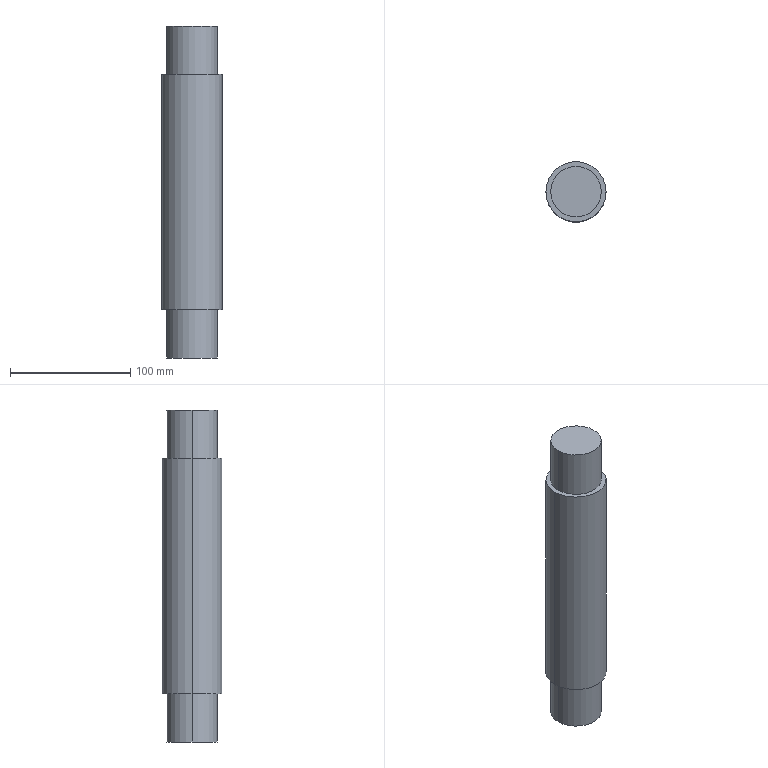Part | SolidWorks | features Extrusion 1, ICE 1, MirrorPattern 1 | 1 solid | 10 faces | box 50 x 50 x 276 mm | volume 495680 mm3 | cylinder 6 | plane 4 | commonest cylinder face diameters 42 x4 50 x2
STEP:
#1=CARTESIAN_POINT('',(21.,0.,-138.));
#2=VERTEX_POINT('',#1);
#3=CARTESIAN_POINT('',(-21.,0.,-138.));
#4=VERTEX_POINT('',#3);
#5=CARTESIAN_POINT('',(0.,0.,-138.));
#6=DIRECTION('',(0.,0.,1.));
#7=DIRECTION('',(1.,0.,0.));
#8=AXIS2_PLACEMENT_3D('',#5,#6,#7);
#9=CIRCLE('',#8,21.);
#10=EDGE_CURVE('',#2,#4,#9,.T.);
#11=ORIENTED_EDGE('',*,*,#10,.T.);
#12=CARTESIAN_POINT('',(-21.,0.,-98.));
#13=VERTEX_POINT('',#12);
#14=CARTESIAN_POINT('',(-21.,0.,-138.));
#15=DIRECTION('',(0.,0.,1.));
#16=VECTOR('',#15,1000.);
#17=LINE('',#14,#16);
#18=EDGE_CURVE('',#4,#13,#17,.T.);
#19=ORIENTED_EDGE('',*,*,#18,.T.);
#20=CARTESIAN_POINT('',(21.,0.,-98.));
#21=VERTEX_POINT('',#20);
#22=CARTESIAN_POINT('',(0.,0.,-98.));
#23=DIRECTION('',(0.,0.,1.));
#24=DIRECTION('',(1.,0.,0.));
#25=AXIS2_PLACEMENT_3D('',#22,#23,#24);
#26=CIRCLE('',#25,21.);
#27=EDGE_CURVE('',#21,#13,#26,.T.);
#28=ORIENTED_EDGE('',*,*,#27,.F.);
#29=CARTESIAN_POINT('',(21.,0.,-138.));
#30=DIRECTION('',(0.,0.,1.));
#31=VECTOR('',#30,1000.);
#32=LINE('',#29,#31);
#33=EDGE_CURVE('',#2,#21,#32,.T.);
#34=ORIENTED_EDGE('',*,*,#33,.F.);
#35=EDGE_LOOP('',(#11,#19,#28,#34));
#36=FACE_OUTER_BOUND('',#35,.T.);
#37=CARTESIAN_POINT('',(0.,0.,-138.));
#38=DIRECTION('',(0.,0.,1.));
#39=DIRECTION('',(1.,0.,0.));
#40=AXIS2_PLACEMENT_3D('',#37,#38,#39);
#41=CYLINDRICAL_SURFACE('',#40,21.);
#42=ADVANCED_FACE('',(#36),#41,.T.);
#43=CARTESIAN_POINT('',(21.,0.,138.));
#44=VERTEX_POINT('',#43);
#45=CARTESIAN_POINT('',(-21.,0.,138.));
#46=VERTEX_POINT('',#45);
#47=CARTESIAN_POINT('',(0.,0.,138.));
#48=DIRECTION('',(0.,0.,1.));
#49=DIRECTION('',(1.,0.,0.));
#50=AXIS2_PLACEMENT_3D('',#47,#48,#49);
#51=CIRCLE('',#50,21.);
#52=EDGE_CURVE('',#44,#46,#51,.T.);
#53=ORIENTED_EDGE('',*,*,#52,.F.);
#54=CARTESIAN_POINT('',(21.,0.,98.));
#55=VERTEX_POINT('',#54);
#56=CARTESIAN_POINT('',(21.,0.,138.));
#57=DIRECTION('',(0.,0.,-1.));
#58=VECTOR('',#57,1000.);
#59=LINE('',#56,#58);
#60=EDGE_CURVE('',#44,#55,#59,.T.);
#61=ORIENTED_EDGE('',*,*,#60,.T.);
#62=CARTESIAN_POINT('',(-21.,0.,98.));
#63=VERTEX_POINT('',#62);
#64=CARTESIAN_POINT('',(0.,0.,98.));
#65=DIRECTION('',(0.,0.,1.));
#66=DIRECTION('',(1.,0.,0.));
#67=AXIS2_PLACEMENT_3D('',#64,#65,#66);
#68=CIRCLE('',#67,21.);
#69=EDGE_CURVE('',#55,#63,#68,.T.);
#70=ORIENTED_EDGE('',*,*,#69,.T.);
#71=CARTESIAN_POINT('',(-21.,0.,138.));
#72=DIRECTION('',(0.,0.,-1.));
#73=VECTOR('',#72,1000.);
#74=LINE('',#71,#73);
#75=EDGE_CURVE('',#46,#63,#74,.T.);
#76=ORIENTED_EDGE('',*,*,#75,.F.);
#77=EDGE_LOOP('',(#53,#61,#70,#76));
#78=FACE_OUTER_BOUND('',#77,.T.);
#79=CARTESIAN_POINT('',(0.,0.,138.));
#80=DIRECTION('',(0.,0.,-1.));
#81=DIRECTION('',(-1.,0.,0.));
#82=AXIS2_PLACEMENT_3D('',#79,#80,#81);
#83=CYLINDRICAL_SURFACE('',#82,21.);
#84=ADVANCED_FACE('',(#78),#83,.T.);
#85=CARTESIAN_POINT('',(25.,0.,98.));
#86=VERTEX_POINT('',#85);
#87=CARTESIAN_POINT('',(-25.,0.,98.));
#88=VERTEX_POINT('',#87);
#89=CARTESIAN_POINT('',(0.,0.,98.));
#90=DIRECTION('',(0.,0.,1.));
#91=DIRECTION('',(1.,0.,0.));
#92=AXIS2_PLACEMENT_3D('',#89,#90,#91);
#93=CIRCLE('',#92,25.);
#94=EDGE_CURVE('',#86,#88,#93,.T.);
#95=ORIENTED_EDGE('',*,*,#94,.F.);
#96=CARTESIAN_POINT('',(25.,0.,-98.));
#97=VERTEX_POINT('',#96);
#98=CARTESIAN_POINT('',(25.,0.,98.));
#99=DIRECTION('',(0.,0.,-1.));
#100=VECTOR('',#99,1000.);
#101=LINE('',#98,#100);
#102=EDGE_CURVE('',#86,#97,#101,.T.);
#103=ORIENTED_EDGE('',*,*,#102,.T.);
#104=CARTESIAN_POINT('',(-25.,0.,-98.));
#105=VERTEX_POINT('',#104);
#106=CARTESIAN_POINT('',(0.,0.,-98.));
#107=DIRECTION('',(0.,0.,1.));
#108=DIRECTION('',(1.,0.,0.));
#109=AXIS2_PLACEMENT_3D('',#106,#107,#108);
#110=CIRCLE('',#109,25.);
#111=EDGE_CURVE('',#97,#105,#110,.T.);
#112=ORIENTED_EDGE('',*,*,#111,.T.);
#113=CARTESIAN_POINT('',(-25.,0.,98.));
#114=DIRECTION('',(0.,0.,-1.));
#115=VECTOR('',#114,1000.);
#116=LINE('',#113,#115);
#117=EDGE_CURVE('',#88,#105,#116,.T.);
#118=ORIENTED_EDGE('',*,*,#117,.F.);
#119=EDGE_LOOP('',(#95,#103,#112,#118));
#120=FACE_OUTER_BOUND('',#119,.T.);
#121=CARTESIAN_POINT('',(0.,0.,98.));
#122=DIRECTION('',(0.,0.,-1.));
#123=DIRECTION('',(-1.,0.,0.));
#124=AXIS2_PLACEMENT_3D('',#121,#122,#123);
#125=CYLINDRICAL_SURFACE('',#124,25.);
#126=ADVANCED_FACE('',(#120),#125,.T.);
#127=ORIENTED_EDGE('',*,*,#102,.F.);
#128=CARTESIAN_POINT('',(0.,0.,98.));
#129=DIRECTION('',(0.,0.,1.));
#130=DIRECTION('',(1.,0.,0.));
#131=AXIS2_PLACEMENT_3D('',#128,#129,#130);
#132=CIRCLE('',#131,25.);
#133=EDGE_CURVE('',#88,#86,#132,.T.);
#134=ORIENTED_EDGE('',*,*,#133,.F.);
#135=ORIENTED_EDGE('',*,*,#117,.T.);
#136=CARTESIAN_POINT('',(0.,0.,-98.));
#137=DIRECTION('',(0.,0.,1.));
#138=DIRECTION('',(1.,0.,0.));
#139=AXIS2_PLACEMENT_3D('',#136,#137,#138);
#140=CIRCLE('',#139,25.);
#141=EDGE_CURVE('',#105,#97,#140,.T.);
#142=ORIENTED_EDGE('',*,*,#141,.T.);
#143=EDGE_LOOP('',(#127,#134,#135,#142));
#144=FACE_OUTER_BOUND('',#143,.T.);
#145=CARTESIAN_POINT('',(0.,0.,98.));
#146=DIRECTION('',(0.,0.,-1.));
#147=DIRECTION('',(-1.,0.,0.));
#148=AXIS2_PLACEMENT_3D('',#145,#146,#147);
#149=CYLINDRICAL_SURFACE('',#148,25.);
#150=ADVANCED_FACE('',(#144),#149,.T.);
#151=CARTESIAN_POINT('',(0.,0.,98.));
#152=DIRECTION('',(0.,0.,1.));
#153=DIRECTION('',(1.,0.,0.));
#154=AXIS2_PLACEMENT_3D('',#151,#152,#153);
#155=CIRCLE('',#154,21.);
#156=EDGE_CURVE('',#63,#55,#155,.T.);
#157=ORIENTED_EDGE('',*,*,#156,.F.);
#158=ORIENTED_EDGE('',*,*,#69,.F.);
#159=EDGE_LOOP('',(#157,#158));
#160=FACE_BOUND('',#159,.T.);
#161=ORIENTED_EDGE('',*,*,#133,.T.);
#162=ORIENTED_EDGE('',*,*,#94,.T.);
#163=EDGE_LOOP('',(#161,#162));
#164=FACE_OUTER_BOUND('',#163,.T.);
#165=CARTESIAN_POINT('',(0.,0.,98.));
#166=DIRECTION('',(0.,0.,1.));
#167=DIRECTION('',(1.,0.,0.));
#168=AXIS2_PLACEMENT_3D('',#165,#166,#167);
#169=PLANE('',#168);
#170=ADVANCED_FACE('',(#160,#164),#169,.T.);
#171=ORIENTED_EDGE('',*,*,#27,.T.);
#172=CARTESIAN_POINT('',(0.,0.,-98.));
#173=DIRECTION('',(0.,0.,1.));
#174=DIRECTION('',(1.,0.,0.));
#175=AXIS2_PLACEMENT_3D('',#172,#173,#174);
#176=CIRCLE('',#175,21.);
#177=EDGE_CURVE('',#13,#21,#176,.T.);
#178=ORIENTED_EDGE('',*,*,#177,.T.);
#179=EDGE_LOOP('',(#171,#178));
#180=FACE_BOUND('',#179,.T.);
#181=ORIENTED_EDGE('',*,*,#141,.F.);
#182=ORIENTED_EDGE('',*,*,#111,.F.);
#183=EDGE_LOOP('',(#181,#182));
#184=FACE_OUTER_BOUND('',#183,.T.);
#185=CARTESIAN_POINT('',(0.,0.,-98.));
#186=DIRECTION('',(0.,0.,1.));
#187=DIRECTION('',(1.,0.,0.));
#188=AXIS2_PLACEMENT_3D('',#185,#186,#187);
#189=PLANE('',#188);
#190=ADVANCED_FACE('',(#180,#184),#189,.F.);
#191=ORIENTED_EDGE('',*,*,#60,.F.);
#192=CARTESIAN_POINT('',(0.,0.,138.));
#193=DIRECTION('',(0.,0.,1.));
#194=DIRECTION('',(1.,0.,0.));
#195=AXIS2_PLACEMENT_3D('',#192,#193,#194);
#196=CIRCLE('',#195,21.);
#197=EDGE_CURVE('',#46,#44,#196,.T.);
#198=ORIENTED_EDGE('',*,*,#197,.F.);
#199=ORIENTED_EDGE('',*,*,#75,.T.);
#200=ORIENTED_EDGE('',*,*,#156,.T.);
#201=EDGE_LOOP('',(#191,#198,#199,#200));
#202=FACE_OUTER_BOUND('',#201,.T.);
#203=CARTESIAN_POINT('',(0.,0.,138.));
#204=DIRECTION('',(0.,0.,-1.));
#205=DIRECTION('',(-1.,0.,0.));
#206=AXIS2_PLACEMENT_3D('',#203,#204,#205);
#207=CYLINDRICAL_SURFACE('',#206,21.);
#208=ADVANCED_FACE('',(#202),#207,.T.);
#209=ORIENTED_EDGE('',*,*,#197,.T.);
#210=ORIENTED_EDGE('',*,*,#52,.T.);
#211=EDGE_LOOP('',(#209,#210));
#212=FACE_OUTER_BOUND('',#211,.T.);
#213=CARTESIAN_POINT('',(0.,0.,138.));
#214=DIRECTION('',(0.,0.,1.));
#215=DIRECTION('',(1.,0.,0.));
#216=AXIS2_PLACEMENT_3D('',#213,#214,#215);
#217=PLANE('',#216);
#218=ADVANCED_FACE('',(#212),#217,.T.);
#219=ORIENTED_EDGE('',*,*,#18,.F.);
#220=CARTESIAN_POINT('',(0.,0.,-138.));
#221=DIRECTION('',(0.,0.,1.));
#222=DIRECTION('',(1.,0.,0.));
#223=AXIS2_PLACEMENT_3D('',#220,#221,#222);
#224=CIRCLE('',#223,21.);
#225=EDGE_CURVE('',#4,#2,#224,.T.);
#226=ORIENTED_EDGE('',*,*,#225,.T.);
#227=ORIENTED_EDGE('',*,*,#33,.T.);
#228=ORIENTED_EDGE('',*,*,#177,.F.);
#229=EDGE_LOOP('',(#219,#226,#227,#228));
#230=FACE_OUTER_BOUND('',#229,.T.);
#231=CARTESIAN_POINT('',(0.,0.,-138.));
#232=DIRECTION('',(0.,0.,1.));
#233=DIRECTION('',(1.,0.,0.));
#234=AXIS2_PLACEMENT_3D('',#231,#232,#233);
#235=CYLINDRICAL_SURFACE('',#234,21.);
#236=ADVANCED_FACE('',(#230),#235,.T.);
#237=ORIENTED_EDGE('',*,*,#10,.F.);
#238=ORIENTED_EDGE('',*,*,#225,.F.);
#239=EDGE_LOOP('',(#237,#238));
#240=FACE_OUTER_BOUND('',#239,.T.);
#241=CARTESIAN_POINT('',(0.,0.,-138.));
#242=DIRECTION('',(0.,0.,-1.));
#243=DIRECTION('',(1.,0.,0.));
#244=AXIS2_PLACEMENT_3D('',#241,#242,#243);
#245=PLANE('',#244);
#246=ADVANCED_FACE('',(#240),#245,.T.);
#247=CLOSED_SHELL('',(#42,#84,#126,#150,#170,#190,#208,#218,#236,#246));
#248=MANIFOLD_SOLID_BREP('',#247);
#249=CARTESIAN_POINT('',(0.,0.,0.));
#250=DIRECTION('',(0.,0.,1.));
#251=DIRECTION('',(1.,0.,0.));
#252=AXIS2_PLACEMENT_3D('',#249,#250,#251);
#253=(LENGTH_UNIT()NAMED_UNIT(*)SI_UNIT(.MILLI.,.METRE.));
#254=UNCERTAINTY_MEASURE_WITH_UNIT(LENGTH_MEASURE(0.00001),#253,'','');
#255=(NAMED_UNIT(*)PLANE_ANGLE_UNIT()SI_UNIT($,.RADIAN.));
#256=(NAMED_UNIT(*)SI_UNIT($,.STERADIAN.)SOLID_ANGLE_UNIT());
#257=(GEOMETRIC_REPRESENTATION_CONTEXT(3)GLOBAL_UNCERTAINTY_ASSIGNED_CONTEXT((#254))GLOBAL_UNIT_ASSIGNED_CONTEXT((#253,#255,#256))REPRESENTATION_CONTEXT('',''));
#258=ADVANCED_BREP_SHAPE_REPRESENTATION('',(#248,#252),#257);